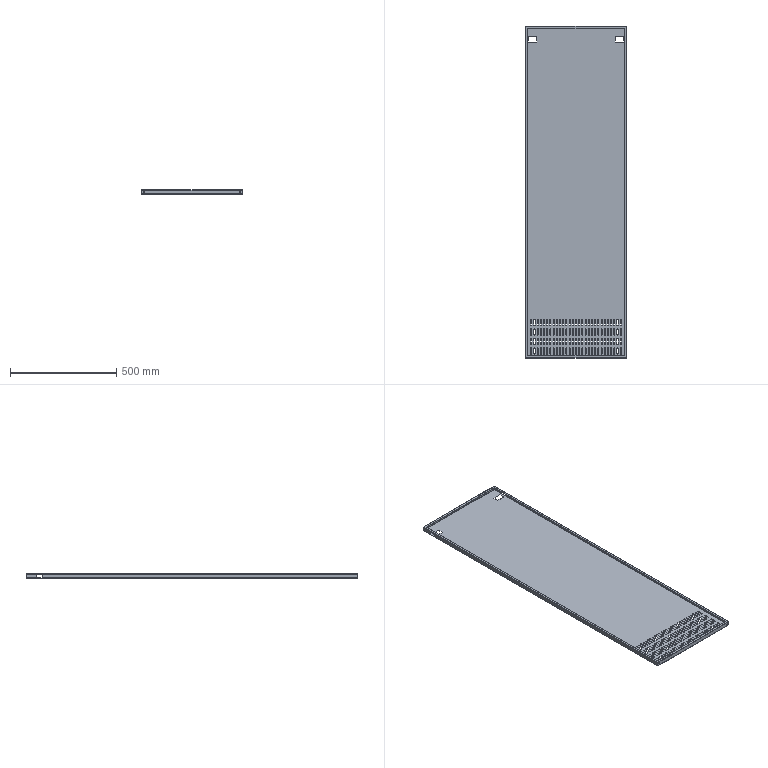Part | SolidWorks | features LPattern 2, ICE 1, SplitBody 1 | 1 solid | 554 faces | box 473 x 1560 x 20 mm | volume 829157 mm3 | plane 284 | cylinder 254 | spline 16 | commonest cylinder face diameters 5 x232 0.2 x10 2.2 x8 4.5 x4